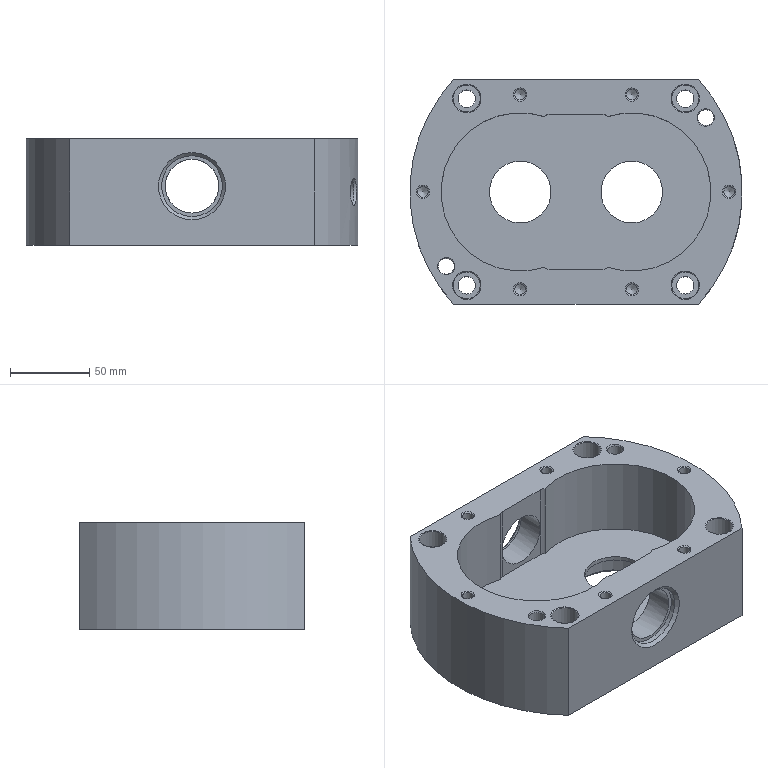NC program | NX | posted with a generic post | part box 210 x 142 x 67.4 mm
Lines 22007 to 22889 of 22889:
(FLOOR_WALL_1_COPY_COPY , TOOL : D12)
N43982 T12 M6
N43984 G54
N43986 G17 G0 G90 X-34.254 Y42.651 B0. C0. S4000 M3
N43988 G43 Z30. H12
N43990 Z-47.2
N43992 G94 G1 Z-50.2 F500.
N43994 G3 X-35.294 Y43.25 R1.2
N43996 G1 X-35.206 F1000.
N43998 G2 X-22.059 Y41.189 R43.25
N44000 G3 X-15.907 Y42.25 R6.75
N44002 G1 X15.907
N44004 G3 X22.059 Y41.189 R6.75
N44006 G2 X35.206 Y43.25 R43.25
N44008 G1 X35.294
N44010 G2 X56.827 Y37.483 R43.25
N44012 G1 X-56.827
N44014 G3 X-64.654 Y31.717 R43.25
N44016 G1 X64.654
N44018 G2 X69.85 Y25.95 R43.25
N44020 G1 X-69.85
N44022 G3 X-73.502 Y20.183 R43.25
N44024 G1 X73.502
N44026 G2 X76.026 Y14.417 R43.25
N44028 G1 X-76.026
N44030 G3 X-77.626 Y8.65 R43.25
N44032 G1 X77.626
N44034 G2 X78.404 Y2.883 R43.25
N44036 G1 X-78.404
N44038 G3 X-78.404 Y-2.883 R43.25
N44040 G1 X78.404
N44042 G2 X77.626 Y-8.65 R43.25
N44044 G1 X-77.626
N44046 G3 X-76.026 Y-14.417 R43.25
N44048 G1 X76.026
N44050 G2 X73.502 Y-20.183 R43.25
N44052 G1 X-73.502
N44054 G3 X-69.85 Y-25.95 R43.25
N44056 G1 X69.85
N44058 G2 X64.654 Y-31.717 R43.25
N44060 G1 X-64.654
N44062 G3 X-56.827 Y-37.483 R43.25
N44064 G1 X56.827
N44066 G2 X35.294 Y-43.25 R43.25
N44068 G1 X35.206
N44070 G2 X34.167 Y-42.65 R1.2
N44072 G1 Z-47.2
N44074 G0 Z30.
N44076 X-34.167
N44078 Z-47.2
N44080 G1 Z-50.2 F500.
N44082 G2 X-35.206 Y-43.25 R1.2
N44084 G1 X-35.294 F1000.
N44086 G2 X-36.333 Y-42.65 R1.2
N44088 G1 Y-43.249
N44090 G3 X-35.295 Y-43.85 R1.2 F500.
N44092 X-21.876 Y-41.761 R43.85 F1000.
N44094 G2 X-16.115 Y-42.85 R6.15
N44096 G1 X16.115
N44098 G2 X21.876 Y-41.761 R6.15
N44100 G3 X21.876 Y41.761 R-43.85
N44102 G2 X16.115 Y42.85 R6.15
N44104 G1 X-16.115
N44106 G2 X-21.876 Y41.761 R6.15
N44108 G3 X-35.295 Y-43.85 R-43.85
N44110 X-34.255 Y-43.251 R1.2
N44112 G1 X-32.824 Y-40.778
N44114 Z-47.2
N44116 G0 Z30.
(ZLEVEL_PROFILE , TOOL : D12)
N44118 X-19.349 Y-35.856 S5000
N44120 Z-14.733
N44122 G1 Z-16.733 F1250.
N44124 X-19.951 Y-37.591
N44126 G3 X-19.724 Y-38.769 R1.2
N44128 G1 X-16.277 Y-42.752
N44130 X-16.063 Y-43.
N44132 X16.063
N44134 X16.277 Y-42.752
N44136 X19.724 Y-38.769
N44138 G3 X19.951 Y-37.591 R1.2
N44140 G1 X19.349 Y-35.855
N44142 Z-14.733
N44144 G0 X-19.349 Z-31.467
N44146 G1 Z-33.467
N44148 X-19.95 Y-37.59
N44150 G3 X-19.724 Y-38.769 R1.2
N44152 G1 X-16.276 Y-42.752
N44154 X-16.062 Y-43.
N44156 X16.062
N44158 X16.694 Y-42.269
N44160 X19.724 Y-38.769
N44162 G3 X19.95 Y-37.59 R1.2
N44164 G1 X19.349 Y-35.855
N44166 Z-31.467
N44168 G0 X-19.348 Z-48.2
N44170 G1 Z-50.2
N44172 X-19.95 Y-37.59
N44174 G3 X-19.723 Y-38.768 R1.2
N44176 G1 X-16.061 Y-43.
N44178 X16.061
N44180 X19.723 Y-38.768
N44182 G3 X19.95 Y-37.59 R1.2
N44184 G1 X19.348 Y-35.855
N44186 Z-48.2
N44188 G0 Z30.
N44190 X19.414 Y35.809
N44192 Z-14.733
N44194 G1 Z-16.733
N44196 X20.006 Y37.532
N44198 G3 X19.775 Y38.71 R1.2
N44200 G1 X19.622 Y38.886
N44202 X16.277 Y42.752
N44204 X16.062 Y43.001
N44206 X16.004 Y43.
N44208 X-16.004
N44210 X-16.062 Y43.001
N44212 X-16.277 Y42.752
N44214 X-19.622 Y38.886
N44216 X-19.775 Y38.71
N44218 G3 X-20.006 Y37.532 R1.2
N44220 G1 X-19.414 Y35.809
N44222 Z-14.733
N44224 G0 X19.413 Y35.81 Z-31.467
N44226 G1 Z-33.467
N44228 X20.005 Y37.532
N44230 G3 X19.775 Y38.71 R1.2
N44232 G1 X19.622 Y38.886
N44234 X16.276 Y42.752
N44236 X16.062 Y43.
N44238 X16.004
N44240 X-16.004
N44242 X-16.062
N44244 X-16.694 Y42.269
N44246 X-19.775 Y38.71
N44248 G3 X-20.002 Y37.531 R1.2
N44250 G1 X-19.406 Y35.814
N44252 Z-31.467
N44254 G0 X19.405 Z-48.2
N44256 G1 Z-50.2
N44258 X20.001 Y37.531
N44260 G3 X19.775 Y38.709 R1.2
N44262 G1 X16.061 Y43.
N44264 X-16.061
N44266 X-19.775 Y38.709
N44268 G3 X-20.001 Y37.531 R1.2
N44270 G1 X-19.405 Y35.814
N44272 Z-48.2
N44274 G0 Z30.
N44276 M5
(HOLE_MILLING_1 , TOOL : D10)
N44278 T10 M6
N44280 G54
N44282 G17 G0 G90 X69. Y-59. B0. C0. S3500 M3
N44284 G43 Z30. H10
N44286 Z0.5
N44288 G94 G3 X70.75 Y-60.75 R1.75 F2200.
N44290 X72.5 Y-59. R1.75
N44292 X72.5 Y-59. Z0.3 I-3.5 J0.
N44294 X72.5 Y-59. Z0.1 I-3.5 J0.
N44296 X72.5 Y-59. Z-0.1 I-3.5 J0.
N44298 X72.5 Y-59. Z-0.3 I-3.5 J0.
N44300 X72.5 Y-59. Z-0.5 I-3.5 J0.
N44302 X72.5 Y-59. Z-0.7 I-3.5 J0.
N44304 X72.5 Y-59. Z-0.9 I-3.5 J0.
N44306 X72.5 Y-59. Z-1.1 I-3.5 J0.
N44308 X72.5 Y-59. Z-1.3 I-3.5 J0.
N44310 X72.5 Y-59. Z-1.5 I-3.5 J0.
N44312 X72.5 Y-59. Z-1.7 I-3.5 J0.
N44314 X72.5 Y-59. Z-1.9 I-3.5 J0.
N44316 X72.5 Y-59. Z-2.1 I-3.5 J0.
N44318 X72.5 Y-59. Z-2.3 I-3.5 J0.
N44320 X72.5 Y-59. Z-2.5 I-3.5 J0.
N44322 X72.5 Y-59. Z-2.7 I-3.5 J0.
N44324 X72.5 Y-59. Z-2.9 I-3.5 J0.
N44326 X72.5 Y-59. Z-3.1 I-3.5 J0.
N44328 X72.5 Y-59. Z-3.3 I-3.5 J0.
N44330 X72.5 Y-59. Z-3.5 I-3.5 J0.
N44332 X72.5 Y-59. Z-3.7 I-3.5 J0.
N44334 X72.5 Y-59. Z-3.9 I-3.5 J0.
N44336 X72.5 Y-59. Z-4.1 I-3.5 J0.
N44338 X72.5 Y-59. Z-4.3 I-3.5 J0.
N44340 X72.5 Y-59. Z-4.5 I-3.5 J0.
N44342 X72.5 Y-59. Z-4.7 I-3.5 J0.
N44344 X72.5 Y-59. Z-4.9 I-3.5 J0.
N44346 X72.5 Y-59. Z-5.1 I-3.5 J0.
N44348 X72.5 Y-59. Z-5.3 I-3.5 J0.
N44350 X72.5 Y-59. Z-5.5 I-3.5 J0.
N44352 X72.5 Y-59. Z-5.7 I-3.5 J0.
N44354 X72.5 Y-59. Z-5.9 I-3.5 J0.
N44356 X72.5 Y-59. Z-6.1 I-3.5 J0.
N44358 X72.5 Y-59. Z-6.3 I-3.5 J0.
N44360 X72.5 Y-59. Z-6.5 I-3.5 J0.
N44362 X72.5 Y-59. Z-6.7 I-3.5 J0.
N44364 X72.5 Y-59. Z-6.9 I-3.5 J0.
N44366 X72.5 Y-59. Z-7.1 I-3.5 J0.
N44368 X72.5 Y-59. Z-7.3 I-3.5 J0.
N44370 X72.5 Y-59. Z-7.5 I-3.5 J0.
N44372 X72.5 Y-59. Z-7.7 I-3.5 J0.
N44374 X72.5 Y-59. Z-7.9 I-3.5 J0.
N44376 X72.5 Y-59. Z-8.1 I-3.5 J0.
N44378 X72.5 Y-59. Z-8.3 I-3.5 J0.
N44380 X72.5 Y-59. Z-8.5 I-3.5 J0.
N44382 X72.5 Y-59. Z-8.7 I-3.5 J0.
N44384 X72.5 Y-59. Z-8.9 I-3.5 J0.
N44386 X72.5 Y-59. Z-9.1 I-3.5 J0.
N44388 X72.5 Y-59. Z-9.3 I-3.5 J0.
N44390 X72.5 Y-59. Z-9.5 I-3.5 J0.
N44392 X72.5 Y-59. Z-9.7 I-3.5 J0.
N44394 X72.5 Y-59. Z-9.9 I-3.5 J0.
N44396 X72.5 Y-59. Z-10.1 I-3.5 J0.
N44398 X72.5 Y-59. Z-10.3 I-3.5 J0.
N44400 X72.5 Y-59. Z-10.5 I-3.5 J0.
N44402 X72.5 Y-59. Z-10.7 I-3.5 J0.
N44404 X72.5 Y-59. Z-10.9 I-3.5 J0.
N44406 X72.5 Y-59. Z-11.1 I-3.5 J0.
N44408 X72.5 Y-59. Z-11.3 I-3.5 J0.
N44410 X72.5 Y-59. Z-11.5 I-3.5 J0.
N44412 X72.5 Y-59. Z-11.7 I-3.5 J0.
N44414 X72.5 Y-59. Z-11.9 I-3.5 J0.
N44416 X72.5 Y-59. Z-12.1 I-3.5 J0.
N44418 X72.5 Y-59. Z-12.3 I-3.5 J0.
N44420 X72.5 Y-59. Z-12.5 I-3.5 J0.
N44422 X72.5 Y-59. Z-12.7 I-3.5 J0.
N44424 X72.5 Y-59. Z-12.9 I-3.5 J0.
N44426 X72.5 Y-59. Z-13.1 I-3.5 J0.
N44428 X72.5 Y-59. Z-13.3 I-3.5 J0.
N44430 X72.5 Y-59. Z-13.5 I-3.5 J0.
N44432 X72.5 Y-59. Z-13.7 I-3.5 J0.
N44434 X72.5 Y-59. Z-13.9 I-3.5 J0.
N44436 X72.5 Y-59. Z-14.1 I-3.5 J0.
N44438 X72.5 Y-59. Z-14.3 I-3.5 J0.
N44440 X72.5 Y-59. Z-14.5 I-3.5 J0.
N44442 X72.5 Y-59. Z-14.7 I-3.5 J0.
N44444 X72.5 Y-59. Z-14.9 I-3.5 J0.
N44446 X72.5 Y-59. Z-15.1 I-3.5 J0.
N44448 X72.5 Y-59. Z-15.3 I-3.5 J0.
N44450 X72.5 Y-59. Z-15.5 I-3.5 J0.
N44452 X72.5 Y-59. Z-15.7 I-3.5 J0.
N44454 X72.5 Y-59. Z-15.9 I-3.5 J0.
N44456 X72.5 Y-59. Z-16.1 I-3.5 J0.
N44458 X72.5 Y-59. Z-16.3 I-3.5 J0.
N44460 X72.5 Y-59. Z-16.5 I-3.5 J0.
N44462 X72.5 Y-59. Z-16.7 I-3.5 J0.
N44464 X72.5 Y-59. Z-16.9 I-3.5 J0.
N44466 X72.5 Y-59. Z-17.1 I-3.5 J0.
N44468 X72.5 Y-59. Z-17.3 I-3.5 J0.
N44470 X72.5 Y-59. Z-17.5 I-3.5 J0.
N44472 X72.5 Y-59. Z-17.7 I-3.5 J0.
N44474 X72.5 Y-59. Z-17.9 I-3.5 J0.
N44476 X72.5 Y-59. Z-18.1 I-3.5 J0.
N44478 X72.5 Y-59. Z-18.3 I-3.5 J0.
N44480 X72.5 Y-59. Z-18.5 I-3.5 J0.
N44482 X72.5 Y-59. Z-18.7 I-3.5 J0.
N44484 X72.5 Y-59. Z-18.9 I-3.5 J0.
N44486 X72.5 Y-59. Z-19.1 I-3.5 J0.
N44488 X72.5 Y-59. Z-19.3 I-3.5 J0.
N44490 X72.5 Y-59. Z-19.5 I-3.5 J0.
N44492 X72.5 Y-59. Z-19.7 I-3.5 J0.
N44494 X72.5 Y-59. Z-19.9 I-3.5 J0.
N44496 X72.5 Y-59. Z-20.1 I-3.5 J0.
N44498 X72.5 Y-59. Z-20.3 I-3.5 J0.
N44500 X72.5 Y-59. Z-20.5 I-3.5 J0.
N44502 X72.5 Y-59. Z-20.7 I-3.5 J0.
N44504 X72.5 Y-59. Z-20.9 I-3.5 J0.
N44506 X72.5 Y-59. Z-21.1 I-3.5 J0.
N44508 X72.5 Y-59. Z-21.3 I-3.5 J0.
N44510 X72.5 Y-59. Z-21.5 I-3.5 J0.
N44512 X72.5 Y-59. Z-21.7 I-3.5 J0.
N44514 X72.5 Y-59. Z-21.9 I-3.5 J0.
N44516 X72.5 Y-59. Z-22.1 I-3.5 J0.
N44518 X72.5 Y-59. Z-22.3 I-3.5 J0.
N44520 X72.5 Y-59. Z-22.5 I-3.5 J0.
N44522 X72.5 Y-59. Z-22.7 I-3.5 J0.
N44524 X72.5 Y-59. Z-22.9 I-3.5 J0.
N44526 X72.5 Y-59. Z-23.1 I-3.5 J0.
N44528 X72.5 Y-59. Z-23.3 I-3.5 J0.
N44530 X72.5 Y-59. Z-23.5 I-3.5 J0.
N44532 X72.5 Y-59. Z-23.7 I-3.5 J0.
N44534 X72.5 Y-59. Z-23.9 I-3.5 J0.
N44536 X72.5 Y-59. Z-24.1 I-3.5 J0.
N44538 X72.5 Y-59. Z-24.3 I-3.5 J0.
N44540 X72.5 Y-59. Z-24.5 I-3.5 J0.
N44542 X72.5 Y-59. Z-24.7 I-3.5 J0.
N44544 X72.5 Y-59. Z-24.9 I-3.5 J0.
N44546 X65.5 Y-59. Z-25. I-3.5 J0.
N44548 X69. Y-62.5 R3.5
N44550 X65.5 Y-59. R-3.5
N44552 X67.25 Y-60.75 R1.75
N44554 X69. Y-59. R1.75
N44556 G0 Z30.
N44558 Y59.
N44560 Z0.5
N44562 G3 X70.75 Y57.25 R1.75
N44564 X72.5 Y59. R1.75
N44566 X72.5 Y59. Z0.3 I-3.5 J0.
N44568 X72.5 Y59. Z0.1 I-3.5 J0.
N44570 X72.5 Y59. Z-0.1 I-3.5 J0.
N44572 X72.5 Y59. Z-0.3 I-3.5 J0.
N44574 X72.5 Y59. Z-0.5 I-3.5 J0.
N44576 X72.5 Y59. Z-0.7 I-3.5 J0.
N44578 X72.5 Y59. Z-0.9 I-3.5 J0.
N44580 X72.5 Y59. Z-1.1 I-3.5 J0.
N44582 X72.5 Y59. Z-1.3 I-3.5 J0.
N44584 X72.5 Y59. Z-1.5 I-3.5 J0.
N44586 X72.5 Y59. Z-1.7 I-3.5 J0.
N44588 X72.5 Y59. Z-1.9 I-3.5 J0.
N44590 X72.5 Y59. Z-2.1 I-3.5 J0.
N44592 X72.5 Y59. Z-2.3 I-3.5 J0.
N44594 X72.5 Y59. Z-2.5 I-3.5 J0.
N44596 X72.5 Y59. Z-2.7 I-3.5 J0.
N44598 X72.5 Y59. Z-2.9 I-3.5 J0.
N44600 X72.5 Y59. Z-3.1 I-3.5 J0.
N44602 X72.5 Y59. Z-3.3 I-3.5 J0.
N44604 X72.5 Y59. Z-3.5 I-3.5 J0.
N44606 X72.5 Y59. Z-3.7 I-3.5 J0.
N44608 X72.5 Y59. Z-3.9 I-3.5 J0.
N44610 X72.5 Y59. Z-4.1 I-3.5 J0.
N44612 X72.5 Y59. Z-4.3 I-3.5 J0.
N44614 X72.5 Y59. Z-4.5 I-3.5 J0.
N44616 X72.5 Y59. Z-4.7 I-3.5 J0.
N44618 X72.5 Y59. Z-4.9 I-3.5 J0.
N44620 X72.5 Y59. Z-5.1 I-3.5 J0.
N44622 X72.5 Y59. Z-5.3 I-3.5 J0.
N44624 X72.5 Y59. Z-5.5 I-3.5 J0.
N44626 X72.5 Y59. Z-5.7 I-3.5 J0.
N44628 X72.5 Y59. Z-5.9 I-3.5 J0.
N44630 X72.5 Y59. Z-6.1 I-3.5 J0.
N44632 X72.5 Y59. Z-6.3 I-3.5 J0.
N44634 X72.5 Y59. Z-6.5 I-3.5 J0.
N44636 X72.5 Y59. Z-6.7 I-3.5 J0.
N44638 X72.5 Y59. Z-6.9 I-3.5 J0.
N44640 X72.5 Y59. Z-7.1 I-3.5 J0.
N44642 X72.5 Y59. Z-7.3 I-3.5 J0.
N44644 X72.5 Y59. Z-7.5 I-3.5 J0.
N44646 X72.5 Y59. Z-7.7 I-3.5 J0.
N44648 X72.5 Y59. Z-7.9 I-3.5 J0.
N44650 X72.5 Y59. Z-8.1 I-3.5 J0.
N44652 X72.5 Y59. Z-8.3 I-3.5 J0.
N44654 X72.5 Y59. Z-8.5 I-3.5 J0.
N44656 X72.5 Y59. Z-8.7 I-3.5 J0.
N44658 X72.5 Y59. Z-8.9 I-3.5 J0.
N44660 X72.5 Y59. Z-9.1 I-3.5 J0.
N44662 X72.5 Y59. Z-9.3 I-3.5 J0.
N44664 X72.5 Y59. Z-9.5 I-3.5 J0.
N44666 X72.5 Y59. Z-9.7 I-3.5 J0.
N44668 X72.5 Y59. Z-9.9 I-3.5 J0.
N44670 X72.5 Y59. Z-10.1 I-3.5 J0.
N44672 X72.5 Y59. Z-10.3 I-3.5 J0.
N44674 X72.5 Y59. Z-10.5 I-3.5 J0.
N44676 X72.5 Y59. Z-10.7 I-3.5 J0.
N44678 X72.5 Y59. Z-10.9 I-3.5 J0.
N44680 X72.5 Y59. Z-11.1 I-3.5 J0.
N44682 X72.5 Y59. Z-11.3 I-3.5 J0.
N44684 X72.5 Y59. Z-11.5 I-3.5 J0.
N44686 X72.5 Y59. Z-11.7 I-3.5 J0.
N44688 X72.5 Y59. Z-11.9 I-3.5 J0.
N44690 X72.5 Y59. Z-12.1 I-3.5 J0.
N44692 X72.5 Y59. Z-12.3 I-3.5 J0.
N44694 X72.5 Y59. Z-12.5 I-3.5 J0.
N44696 X72.5 Y59. Z-12.7 I-3.5 J0.
N44698 X72.5 Y59. Z-12.9 I-3.5 J0.
N44700 X72.5 Y59. Z-13.1 I-3.5 J0.
N44702 X72.5 Y59. Z-13.3 I-3.5 J0.
N44704 X72.5 Y59. Z-13.5 I-3.5 J0.
N44706 X72.5 Y59. Z-13.7 I-3.5 J0.
N44708 X72.5 Y59. Z-13.9 I-3.5 J0.
N44710 X72.5 Y59. Z-14.1 I-3.5 J0.
N44712 X72.5 Y59. Z-14.3 I-3.5 J0.
N44714 X72.5 Y59. Z-14.5 I-3.5 J0.
N44716 X72.5 Y59. Z-14.7 I-3.5 J0.
N44718 X72.5 Y59. Z-14.9 I-3.5 J0.
N44720 X72.5 Y59. Z-15.1 I-3.5 J0.
N44722 X72.5 Y59. Z-15.3 I-3.5 J0.
N44724 X72.5 Y59. Z-15.5 I-3.5 J0.
N44726 X72.5 Y59. Z-15.7 I-3.5 J0.
N44728 X72.5 Y59. Z-15.9 I-3.5 J0.
N44730 X72.5 Y59. Z-16.1 I-3.5 J0.
N44732 X72.5 Y59. Z-16.3 I-3.5 J0.
N44734 X72.5 Y59. Z-16.5 I-3.5 J0.
N44736 X72.5 Y59. Z-16.7 I-3.5 J0.
N44738 X72.5 Y59. Z-16.9 I-3.5 J0.
N44740 X72.5 Y59. Z-17.1 I-3.5 J0.
N44742 X72.5 Y59. Z-17.3 I-3.5 J0.
N44744 X72.5 Y59. Z-17.5 I-3.5 J0.
N44746 X72.5 Y59. Z-17.7 I-3.5 J0.
N44748 X72.5 Y59. Z-17.9 I-3.5 J0.
N44750 X72.5 Y59. Z-18.1 I-3.5 J0.
N44752 X72.5 Y59. Z-18.3 I-3.5 J0.
N44754 X72.5 Y59. Z-18.5 I-3.5 J0.
N44756 X72.5 Y59. Z-18.7 I-3.5 J0.
N44758 X72.5 Y59. Z-18.9 I-3.5 J0.
N44760 X72.5 Y59. Z-19.1 I-3.5 J0.
N44762 X72.5 Y59. Z-19.3 I-3.5 J0.
N44764 X72.5 Y59. Z-19.5 I-3.5 J0.
N44766 X72.5 Y59. Z-19.7 I-3.5 J0.
N44768 X72.5 Y59. Z-19.9 I-3.5 J0.
N44770 X72.5 Y59. Z-20.1 I-3.5 J0.
N44772 X72.5 Y59. Z-20.3 I-3.5 J0.
N44774 X72.5 Y59. Z-20.5 I-3.5 J0.
N44776 X72.5 Y59. Z-20.7 I-3.5 J0.
N44778 X72.5 Y59. Z-20.9 I-3.5 J0.
N44780 X72.5 Y59. Z-21.1 I-3.5 J0.
N44782 X72.5 Y59. Z-21.3 I-3.5 J0.
N44784 X72.5 Y59. Z-21.5 I-3.5 J0.
N44786 X72.5 Y59. Z-21.7 I-3.5 J0.
N44788 X72.5 Y59. Z-21.9 I-3.5 J0.
N44790 X72.5 Y59. Z-22.1 I-3.5 J0.
N44792 X72.5 Y59. Z-22.3 I-3.5 J0.
N44794 X72.5 Y59. Z-22.5 I-3.5 J0.
N44796 X72.5 Y59. Z-22.7 I-3.5 J0.
N44798 X72.5 Y59. Z-22.9 I-3.5 J0.
N44800 X72.5 Y59. Z-23.1 I-3.5 J0.
N44802 X72.5 Y59. Z-23.3 I-3.5 J0.
N44804 X72.5 Y59. Z-23.5 I-3.5 J0.
N44806 X72.5 Y59. Z-23.7 I-3.5 J0.
N44808 X72.5 Y59. Z-23.9 I-3.5 J0.
N44810 X72.5 Y59. Z-24.1 I-3.5 J0.
N44812 X72.5 Y59. Z-24.3 I-3.5 J0.
N44814 X72.5 Y59. Z-24.5 I-3.5 J0.
N44816 X72.5 Y59. Z-24.7 I-3.5 J0.
N44818 X72.5 Y59. Z-24.9 I-3.5 J0.
N44820 X65.5 Y59. Z-25. I-3.5 J0.
N44822 X69. Y55.5 R3.5
N44824 X65.5 Y59. R-3.5
N44826 X67.25 Y57.25 R1.75
N44828 X69. Y59. R1.75
N44830 G0 Z30.
N44832 X-69.
N44834 Z0.5
N44836 G3 X-67.25 Y57.25 R1.75
N44838 X-65.5 Y59. R1.75
N44840 X-65.5 Y59. Z0.3 I-3.5 J0.
N44842 X-65.5 Y59. Z0.1 I-3.5 J0.
N44844 X-65.5 Y59. Z-0.1 I-3.5 J0.
N44846 X-65.5 Y59. Z-0.3 I-3.5 J0.
N44848 X-65.5 Y59. Z-0.5 I-3.5 J0.
N44850 X-65.5 Y59. Z-0.7 I-3.5 J0.
N44852 X-65.5 Y59. Z-0.9 I-3.5 J0.
N44854 X-65.5 Y59. Z-1.1 I-3.5 J0.
N44856 X-65.5 Y59. Z-1.3 I-3.5 J0.
N44858 X-65.5 Y59. Z-1.5 I-3.5 J0.
N44860 X-65.5 Y59. Z-1.7 I-3.5 J0.
N44862 X-65.5 Y59. Z-1.9 I-3.5 J0.
N44864 X-65.5 Y59. Z-2.1 I-3.5 J0.
N44866 X-65.5 Y59. Z-2.3 I-3.5 J0.
N44868 X-65.5 Y59. Z-2.5 I-3.5 J0.
N44870 X-65.5 Y59. Z-2.7 I-3.5 J0.
N44872 X-65.5 Y59. Z-2.9 I-3.5 J0.
N44874 X-65.5 Y59. Z-3.1 I-3.5 J0.
N44876 X-65.5 Y59. Z-3.3 I-3.5 J0.
N44878 X-65.5 Y59. Z-3.5 I-3.5 J0.
N44880 X-65.5 Y59. Z-3.7 I-3.5 J0.
N44882 X-65.5 Y59. Z-3.9 I-3.5 J0.
N44884 X-65.5 Y59. Z-4.1 I-3.5 J0.
N44886 X-65.5 Y59. Z-4.3 I-3.5 J0.
N44888 X-65.5 Y59. Z-4.5 I-3.5 J0.
N44890 X-65.5 Y59. Z-4.7 I-3.5 J0.
N44892 X-65.5 Y59. Z-4.9 I-3.5 J0.
N44894 X-65.5 Y59. Z-5.1 I-3.5 J0.
N44896 X-65.5 Y59. Z-5.3 I-3.5 J0.
N44898 X-65.5 Y59. Z-5.5 I-3.5 J0.
N44900 X-65.5 Y59. Z-5.7 I-3.5 J0.
N44902 X-65.5 Y59. Z-5.9 I-3.5 J0.
N44904 X-65.5 Y59. Z-6.1 I-3.5 J0.
N44906 X-65.5 Y59. Z-6.3 I-3.5 J0.
N44908 X-65.5 Y59. Z-6.5 I-3.5 J0.
N44910 X-65.5 Y59. Z-6.7 I-3.5 J0.
N44912 X-65.5 Y59. Z-6.9 I-3.5 J0.
N44914 X-65.5 Y59. Z-7.1 I-3.5 J0.
N44916 X-65.5 Y59. Z-7.3 I-3.5 J0.
N44918 X-65.5 Y59. Z-7.5 I-3.5 J0.
N44920 X-65.5 Y59. Z-7.7 I-3.5 J0.
N44922 X-65.5 Y59. Z-7.9 I-3.5 J0.
N44924 X-65.5 Y59. Z-8.1 I-3.5 J0.
N44926 X-65.5 Y59. Z-8.3 I-3.5 J0.
N44928 X-65.5 Y59. Z-8.5 I-3.5 J0.
N44930 X-65.5 Y59. Z-8.7 I-3.5 J0.
N44932 X-65.5 Y59. Z-8.9 I-3.5 J0.
N44934 X-65.5 Y59. Z-9.1 I-3.5 J0.
N44936 X-65.5 Y59. Z-9.3 I-3.5 J0.
N44938 X-65.5 Y59. Z-9.5 I-3.5 J0.
N44940 X-65.5 Y59. Z-9.7 I-3.5 J0.
N44942 X-65.5 Y59. Z-9.9 I-3.5 J0.
N44944 X-65.5 Y59. Z-10.1 I-3.5 J0.
N44946 X-65.5 Y59. Z-10.3 I-3.5 J0.
N44948 X-65.5 Y59. Z-10.5 I-3.5 J0.
N44950 X-65.5 Y59. Z-10.7 I-3.5 J0.
N44952 X-65.5 Y59. Z-10.9 I-3.5 J0.
N44954 X-65.5 Y59. Z-11.1 I-3.5 J0.
N44956 X-65.5 Y59. Z-11.3 I-3.5 J0.
N44958 X-65.5 Y59. Z-11.5 I-3.5 J0.
N44960 X-65.5 Y59. Z-11.7 I-3.5 J0.
N44962 X-65.5 Y59. Z-11.9 I-3.5 J0.
N44964 X-65.5 Y59. Z-12.1 I-3.5 J0.
N44966 X-65.5 Y59. Z-12.3 I-3.5 J0.
N44968 X-65.5 Y59. Z-12.5 I-3.5 J0.
N44970 X-65.5 Y59. Z-12.7 I-3.5 J0.
N44972 X-65.5 Y59. Z-12.9 I-3.5 J0.
N44974 X-65.5 Y59. Z-13.1 I-3.5 J0.
N44976 X-65.5 Y59. Z-13.3 I-3.5 J0.
N44978 X-65.5 Y59. Z-13.5 I-3.5 J0.
N44980 X-65.5 Y59. Z-13.7 I-3.5 J0.
N44982 X-65.5 Y59. Z-13.9 I-3.5 J0.
N44984 X-65.5 Y59. Z-14.1 I-3.5 J0.
N44986 X-65.5 Y59. Z-14.3 I-3.5 J0.
N44988 X-65.5 Y59. Z-14.5 I-3.5 J0.
N44990 X-65.5 Y59. Z-14.7 I-3.5 J0.
N44992 X-65.5 Y59. Z-14.9 I-3.5 J0.
N44994 X-65.5 Y59. Z-15.1 I-3.5 J0.
N44996 X-65.5 Y59. Z-15.3 I-3.5 J0.
N44998 X-65.5 Y59. Z-15.5 I-3.5 J0.
N45000 X-65.5 Y59. Z-15.7 I-3.5 J0.
N45002 X-65.5 Y59. Z-15.9 I-3.5 J0.
N45004 X-65.5 Y59. Z-16.1 I-3.5 J0.
N45006 X-65.5 Y59. Z-16.3 I-3.5 J0.
N45008 X-65.5 Y59. Z-16.5 I-3.5 J0.
N45010 X-65.5 Y59. Z-16.7 I-3.5 J0.
N45012 X-65.5 Y59. Z-16.9 I-3.5 J0.
N45014 X-65.5 Y59. Z-17.1 I-3.5 J0.
N45016 X-65.5 Y59. Z-17.3 I-3.5 J0.
N45018 X-65.5 Y59. Z-17.5 I-3.5 J0.
N45020 X-65.5 Y59. Z-17.7 I-3.5 J0.
N45022 X-65.5 Y59. Z-17.9 I-3.5 J0.
N45024 X-65.5 Y59. Z-18.1 I-3.5 J0.
N45026 X-65.5 Y59. Z-18.3 I-3.5 J0.
N45028 X-65.5 Y59. Z-18.5 I-3.5 J0.
N45030 X-65.5 Y59. Z-18.7 I-3.5 J0.
N45032 X-65.5 Y59. Z-18.9 I-3.5 J0.
N45034 X-65.5 Y59. Z-19.1 I-3.5 J0.
N45036 X-65.5 Y59. Z-19.3 I-3.5 J0.
N45038 X-65.5 Y59. Z-19.5 I-3.5 J0.
N45040 X-65.5 Y59. Z-19.7 I-3.5 J0.
N45042 X-65.5 Y59. Z-19.9 I-3.5 J0.
N45044 X-65.5 Y59. Z-20.1 I-3.5 J0.
N45046 X-65.5 Y59. Z-20.3 I-3.5 J0.
N45048 X-65.5 Y59. Z-20.5 I-3.5 J0.
N45050 X-65.5 Y59. Z-20.7 I-3.5 J0.
N45052 X-65.5 Y59. Z-20.9 I-3.5 J0.
N45054 X-65.5 Y59. Z-21.1 I-3.5 J0.
N45056 X-65.5 Y59. Z-21.3 I-3.5 J0.
N45058 X-65.5 Y59. Z-21.5 I-3.5 J0.
N45060 X-65.5 Y59. Z-21.7 I-3.5 J0.
N45062 X-65.5 Y59. Z-21.9 I-3.5 J0.
N45064 X-65.5 Y59. Z-22.1 I-3.5 J0.
N45066 X-65.5 Y59. Z-22.3 I-3.5 J0.
N45068 X-65.5 Y59. Z-22.5 I-3.5 J0.
N45070 X-65.5 Y59. Z-22.7 I-3.5 J0.
N45072 X-65.5 Y59. Z-22.9 I-3.5 J0.
N45074 X-65.5 Y59. Z-23.1 I-3.5 J0.
N45076 X-65.5 Y59. Z-23.3 I-3.5 J0.
N45078 X-65.5 Y59. Z-23.5 I-3.5 J0.
N45080 X-65.5 Y59. Z-23.7 I-3.5 J0.
N45082 X-65.5 Y59. Z-23.9 I-3.5 J0.
N45084 X-65.5 Y59. Z-24.1 I-3.5 J0.
N45086 X-65.5 Y59. Z-24.3 I-3.5 J0.
N45088 X-65.5 Y59. Z-24.5 I-3.5 J0.
N45090 X-65.5 Y59. Z-24.7 I-3.5 J0.
N45092 X-65.5 Y59. Z-24.9 I-3.5 J0.
N45094 X-72.5 Y59. Z-25. I-3.5 J0.
N45096 X-69. Y55.5 R3.5
N45098 X-72.5 Y59. R-3.5
N45100 X-70.75 Y57.25 R1.75
N45102 X-69. Y59. R1.75
N45104 G0 Z30.
N45106 Y-59.
N45108 Z0.5
N45110 G3 X-67.25 Y-60.75 R1.75
N45112 X-65.5 Y-59. R1.75
N45114 X-65.5 Y-59. Z0.3 I-3.5 J0.
N45116 X-65.5 Y-59. Z0.1 I-3.5 J0.
N45118 X-65.5 Y-59. Z-0.1 I-3.5 J0.
N45120 X-65.5 Y-59. Z-0.3 I-3.5 J0.
N45122 X-65.5 Y-59. Z-0.5 I-3.5 J0.
N45124 X-65.5 Y-59. Z-0.7 I-3.5 J0.
N45126 X-65.5 Y-59. Z-0.9 I-3.5 J0.
N45128 X-65.5 Y-59. Z-1.1 I-3.5 J0.
N45130 X-65.5 Y-59. Z-1.3 I-3.5 J0.
N45132 X-65.5 Y-59. Z-1.5 I-3.5 J0.
N45134 X-65.5 Y-59. Z-1.7 I-3.5 J0.
N45136 X-65.5 Y-59. Z-1.9 I-3.5 J0.
N45138 X-65.5 Y-59. Z-2.1 I-3.5 J0.
N45140 X-65.5 Y-59. Z-2.3 I-3.5 J0.
N45142 X-65.5 Y-59. Z-2.5 I-3.5 J0.
N45144 X-65.5 Y-59. Z-2.7 I-3.5 J0.
N45146 X-65.5 Y-59. Z-2.9 I-3.5 J0.
N45148 X-65.5 Y-59. Z-3.1 I-3.5 J0.
N45150 X-65.5 Y-59. Z-3.3 I-3.5 J0.
N45152 X-65.5 Y-59. Z-3.5 I-3.5 J0.
N45154 X-65.5 Y-59. Z-3.7 I-3.5 J0.
N45156 X-65.5 Y-59. Z-3.9 I-3.5 J0.
N45158 X-65.5 Y-59. Z-4.1 I-3.5 J0.
N45160 X-65.5 Y-59. Z-4.3 I-3.5 J0.
N45162 X-65.5 Y-59. Z-4.5 I-3.5 J0.
N45164 X-65.5 Y-59. Z-4.7 I-3.5 J0.
N45166 X-65.5 Y-59. Z-4.9 I-3.5 J0.
N45168 X-65.5 Y-59. Z-5.1 I-3.5 J0.
N45170 X-65.5 Y-59. Z-5.3 I-3.5 J0.
N45172 X-65.5 Y-59. Z-5.5 I-3.5 J0.
N45174 X-65.5 Y-59. Z-5.7 I-3.5 J0.
N45176 X-65.5 Y-59. Z-5.9 I-3.5 J0.
N45178 X-65.5 Y-59. Z-6.1 I-3.5 J0.
N45180 X-65.5 Y-59. Z-6.3 I-3.5 J0.
N45182 X-65.5 Y-59. Z-6.5 I-3.5 J0.
N45184 X-65.5 Y-59. Z-6.7 I-3.5 J0.
N45186 X-65.5 Y-59. Z-6.9 I-3.5 J0.
N45188 X-65.5 Y-59. Z-7.1 I-3.5 J0.
N45190 X-65.5 Y-59. Z-7.3 I-3.5 J0.
N45192 X-65.5 Y-59. Z-7.5 I-3.5 J0.
N45194 X-65.5 Y-59. Z-7.7 I-3.5 J0.
N45196 X-65.5 Y-59. Z-7.9 I-3.5 J0.
N45198 X-65.5 Y-59. Z-8.1 I-3.5 J0.
N45200 X-65.5 Y-59. Z-8.3 I-3.5 J0.
N45202 X-65.5 Y-59. Z-8.5 I-3.5 J0.
N45204 X-65.5 Y-59. Z-8.7 I-3.5 J0.
N45206 X-65.5 Y-59. Z-8.9 I-3.5 J0.
N45208 X-65.5 Y-59. Z-9.1 I-3.5 J0.
N45210 X-65.5 Y-59. Z-9.3 I-3.5 J0.
N45212 X-65.5 Y-59. Z-9.5 I-3.5 J0.
N45214 X-65.5 Y-59. Z-9.7 I-3.5 J0.
N45216 X-65.5 Y-59. Z-9.9 I-3.5 J0.
N45218 X-65.5 Y-59. Z-10.1 I-3.5 J0.
N45220 X-65.5 Y-59. Z-10.3 I-3.5 J0.
N45222 X-65.5 Y-59. Z-10.5 I-3.5 J0.
N45224 X-65.5 Y-59. Z-10.7 I-3.5 J0.
N45226 X-65.5 Y-59. Z-10.9 I-3.5 J0.
N45228 X-65.5 Y-59. Z-11.1 I-3.5 J0.
N45230 X-65.5 Y-59. Z-11.3 I-3.5 J0.
N45232 X-65.5 Y-59. Z-11.5 I-3.5 J0.
N45234 X-65.5 Y-59. Z-11.7 I-3.5 J0.
N45236 X-65.5 Y-59. Z-11.9 I-3.5 J0.
N45238 X-65.5 Y-59. Z-12.1 I-3.5 J0.
N45240 X-65.5 Y-59. Z-12.3 I-3.5 J0.
N45242 X-65.5 Y-59. Z-12.5 I-3.5 J0.
N45244 X-65.5 Y-59. Z-12.7 I-3.5 J0.
N45246 X-65.5 Y-59. Z-12.9 I-3.5 J0.
N45248 X-65.5 Y-59. Z-13.1 I-3.5 J0.
N45250 X-65.5 Y-59. Z-13.3 I-3.5 J0.
N45252 X-65.5 Y-59. Z-13.5 I-3.5 J0.
N45254 X-65.5 Y-59. Z-13.7 I-3.5 J0.
N45256 X-65.5 Y-59. Z-13.9 I-3.5 J0.
N45258 X-65.5 Y-59. Z-14.1 I-3.5 J0.
N45260 X-65.5 Y-59. Z-14.3 I-3.5 J0.
N45262 X-65.5 Y-59. Z-14.5 I-3.5 J0.
N45264 X-65.5 Y-59. Z-14.7 I-3.5 J0.
N45266 X-65.5 Y-59. Z-14.9 I-3.5 J0.
N45268 X-65.5 Y-59. Z-15.1 I-3.5 J0.
N45270 X-65.5 Y-59. Z-15.3 I-3.5 J0.
N45272 X-65.5 Y-59. Z-15.5 I-3.5 J0.
N45274 X-65.5 Y-59. Z-15.7 I-3.5 J0.
N45276 X-65.5 Y-59. Z-15.9 I-3.5 J0.
N45278 X-65.5 Y-59. Z-16.1 I-3.5 J0.
N45280 X-65.5 Y-59. Z-16.3 I-3.5 J0.
N45282 X-65.5 Y-59. Z-16.5 I-3.5 J0.
N45284 X-65.5 Y-59. Z-16.7 I-3.5 J0.
N45286 X-65.5 Y-59. Z-16.9 I-3.5 J0.
N45288 X-65.5 Y-59. Z-17.1 I-3.5 J0.
N45290 X-65.5 Y-59. Z-17.3 I-3.5 J0.
N45292 X-65.5 Y-59. Z-17.5 I-3.5 J0.
N45294 X-65.5 Y-59. Z-17.7 I-3.5 J0.
N45296 X-65.5 Y-59. Z-17.9 I-3.5 J0.
N45298 X-65.5 Y-59. Z-18.1 I-3.5 J0.
N45300 X-65.5 Y-59. Z-18.3 I-3.5 J0.
N45302 X-65.5 Y-59. Z-18.5 I-3.5 J0.
N45304 X-65.5 Y-59. Z-18.7 I-3.5 J0.
N45306 X-65.5 Y-59. Z-18.9 I-3.5 J0.
N45308 X-65.5 Y-59. Z-19.1 I-3.5 J0.
N45310 X-65.5 Y-59. Z-19.3 I-3.5 J0.
N45312 X-65.5 Y-59. Z-19.5 I-3.5 J0.
N45314 X-65.5 Y-59. Z-19.7 I-3.5 J0.
N45316 X-65.5 Y-59. Z-19.9 I-3.5 J0.
N45318 X-65.5 Y-59. Z-20.1 I-3.5 J0.
N45320 X-65.5 Y-59. Z-20.3 I-3.5 J0.
N45322 X-65.5 Y-59. Z-20.5 I-3.5 J0.
N45324 X-65.5 Y-59. Z-20.7 I-3.5 J0.
N45326 X-65.5 Y-59. Z-20.9 I-3.5 J0.
N45328 X-65.5 Y-59. Z-21.1 I-3.5 J0.
N45330 X-65.5 Y-59. Z-21.3 I-3.5 J0.
N45332 X-65.5 Y-59. Z-21.5 I-3.5 J0.
N45334 X-65.5 Y-59. Z-21.7 I-3.5 J0.
N45336 X-65.5 Y-59. Z-21.9 I-3.5 J0.
N45338 X-65.5 Y-59. Z-22.1 I-3.5 J0.
N45340 X-65.5 Y-59. Z-22.3 I-3.5 J0.
N45342 X-65.5 Y-59. Z-22.5 I-3.5 J0.
N45344 X-65.5 Y-59. Z-22.7 I-3.5 J0.
N45346 X-65.5 Y-59. Z-22.9 I-3.5 J0.
N45348 X-65.5 Y-59. Z-23.1 I-3.5 J0.
N45350 X-65.5 Y-59. Z-23.3 I-3.5 J0.
N45352 X-65.5 Y-59. Z-23.5 I-3.5 J0.
N45354 X-65.5 Y-59. Z-23.7 I-3.5 J0.
N45356 X-65.5 Y-59. Z-23.9 I-3.5 J0.
N45358 X-65.5 Y-59. Z-24.1 I-3.5 J0.
N45360 X-65.5 Y-59. Z-24.3 I-3.5 J0.
N45362 X-65.5 Y-59. Z-24.5 I-3.5 J0.
N45364 X-65.5 Y-59. Z-24.7 I-3.5 J0.
N45366 X-65.5 Y-59. Z-24.9 I-3.5 J0.
N45368 X-72.5 Y-59. Z-25. I-3.5 J0.
N45370 X-69. Y-62.5 R3.5
N45372 X-72.5 Y-59. R-3.5
N45374 X-70.75 Y-60.75 R1.75
N45376 X-69. Y-59. R1.75
N45378 G0 Z30.
N45380 M5
(PLANAR_MILL_COPY_1_COPY_1 , TOOL : D6A45)
N45382 T07 M6
N45384 G54
N45386 G17 G0 G90 X-1.473 Y-47.3 B0. C0. S7500 M3
N45388 G43 Z30. H7
N45390 Z2.
N45392 G94 G1 Z-1. F1250.
N45394 X-0.766 Y-48.143
N45396 G3 X0. Y-48.5 R1.
N45398 G1 X16.975
N45400 G3 X19.444 Y-47.481 R3.5
N45402 G2 X20.449 Y-47.235 R1.
N45404 G3 X20.449 Y47.235 R-49.5
N45406 G2 X19.444 Y47.481 R1.
N45408 G3 X16.975 Y48.5 R3.5
N45410 G1 X-16.975
N45412 G3 X-19.444 Y47.481 R3.5
N45414 G2 X-20.449 Y47.235 R1.
N45416 G3 X-20.449 Y-47.235 R-49.5
N45418 G2 X-19.444 Y-47.481 R1.
N45420 G3 X-16.975 Y-48.5 R3.5
N45422 G1 X0.
N45424 G3 X0.766 Y-48.143 R1.
N45426 G1 X1.473 Y-47.3
N45428 Z2.
N45430 G0 Z30.
N45432 X-34.76 Y63.128
N45434 Z2.
N45436 G1 Z-1.
N45438 X-34.484 Y64.043
N45440 G3 X-35.25 Y64.4 R1.
N45442 X-38.15 Y61.5 R2.9
N45444 X-35.25 Y64.4 R-2.9
N45446 X-36.016 Y64.043 R1.
N45448 G1 X-35.74 Y63.128
N45450 Z2.
N45452 G0 Z30.
N45454 X-67.358 Y65.599
N45456 Z2.
N45458 G1 Z-1.
N45460 X-68.234 Y66.643
N45462 G3 X-69. Y67. R1.
N45464 X-77. Y59. R8.
N45466 X-69. Y67. R-8.
N45468 X-69.766 Y66.643 R1.
N45470 G1 X-70.642 Y65.599
N45472 Z2.
N45474 G0 Z30.
N45476 X-98.378 Y0.49
N45478 Z2.
N45480 G1 Z-1.
N45482 X-99.293 Y0.766
N45484 G3 X-99.65 Y0. R1.
N45486 X-96.75 Y-2.9 R2.9
N45488 X-99.65 Y0. R-2.9
N45490 X-99.293 Y-0.766 R1.
N45492 G1 X-98.378 Y-0.49
N45494 Z2.
N45496 G0 Z30.
N45498 X-84.528 Y-44.879
N45500 Z2.
N45502 G1 Z-1.
N45504 X-86.143 Y-46.234
N45506 G3 X-86.5 Y-47. R1.
N45508 X-82. Y-51.5 R4.5
N45510 X-86.5 Y-47. R-4.5
N45512 X-86.143 Y-47.766 R1.
N45514 G1 X-84.528 Y-49.121
N45516 Z2.
N45518 G0 Z30.
N45520 X-70.642 Y-65.599
N45522 Z2.
N45524 G1 Z-1.
N45526 X-69.766 Y-66.643
N45528 G3 X-69. Y-67. R1.
N45530 X-61. Y-59. R8.
N45532 X-69. Y-67. R-8.
N45534 X-68.234 Y-66.643 R1.
N45536 G1 X-67.358 Y-65.599
N45538 Z2.
N45540 G0 Z30.
N45542 X-35.74 Y-63.128
N45544 Z2.
N45546 G1 Z-1.
N45548 X-36.016 Y-64.043
N45550 G3 X-35.25 Y-64.4 R1.
N45552 X-32.35 Y-61.5 R2.9
N45554 X-35.25 Y-64.4 R-2.9
N45556 X-34.484 Y-64.043 R1.
N45558 G1 X-34.76 Y-63.128
N45560 Z2.
N45562 G0 Z30.
N45564 X34.76
N45566 Z2.
N45568 G1 Z-1.
N45570 X34.484 Y-64.043
N45572 G3 X35.25 Y-64.4 R1.
N45574 X38.15 Y-61.5 R2.9
N45576 X35.25 Y-64.4 R-2.9
N45578 X36.016 Y-64.043 R1.
N45580 G1 X35.74 Y-63.128
N45582 Z2.
N45584 G0 Z30.
N45586 X67.358 Y-65.599
N45588 Z2.
N45590 G1 Z-1.
N45592 X68.234 Y-66.643
N45594 G3 X69. Y-67. R1.
N45596 X77. Y-59. R8.
N45598 X69. Y-67. R-8.
N45600 X69.766 Y-66.643 R1.
N45602 G1 X70.642 Y-65.599
N45604 Z2.
N45606 G0 Z30.
N45608 X98.378 Y-0.49
N45610 Z2.
N45612 G1 Z-1.
N45614 X99.293 Y-0.766
N45616 G3 X99.65 Y0. R1.
N45618 X96.75 Y2.9 R2.9
N45620 X99.65 Y0. R-2.9
N45622 X99.293 Y0.766 R1.
N45624 G1 X98.378 Y0.49
N45626 Z2.
N45628 G0 Z30.
N45630 X84.528 Y44.879
N45632 Z2.
N45634 G1 Z-1.
N45636 X86.143 Y46.234
N45638 G3 X86.5 Y47. R1.
N45640 X82. Y51.5 R4.5
N45642 X86.5 Y47. R-4.5
N45644 X86.143 Y47.766 R1.
N45646 G1 X84.528 Y49.121
N45648 Z2.
N45650 G0 Z30.
N45652 X70.642 Y65.599
N45654 Z2.
N45656 G1 Z-1.
N45658 X69.766 Y66.643
N45660 G3 X69. Y67. R1.
N45662 X61. Y59. R8.
N45664 X69. Y67. R-8.
N45666 X68.234 Y66.643 R1.
N45668 G1 X67.358 Y65.599
N45670 Z2.
N45672 G0 Z30.
N45674 X35.74 Y63.128
N45676 Z2.
N45678 G1 Z-1.
N45680 X36.016 Y64.043
N45682 G3 X35.25 Y64.4 R1.
N45684 X32.35 Y61.5 R2.9
N45686 X35.25 Y64.4 R-2.9
N45688 X34.484 Y64.043 R1.
N45690 G1 X34.76 Y63.128
N45692 Z2.
N45694 G0 Z30.
N45696 M5
(DRILLING_1 , TOOL : D100JD)
N45698 T24 M6
N45700 G54
N45702 G17 G0 G90 X-35.25 Y0. B0. C0. S300 M3
N45704 G43 Z30. H24
N45706 G94 G85 G98 Z-50.2 F50. R3.
N45708 X35.25
N45710 G80
N45712 G0 X35.25 Y0. Z30.
N45714 M5
N45716 M2